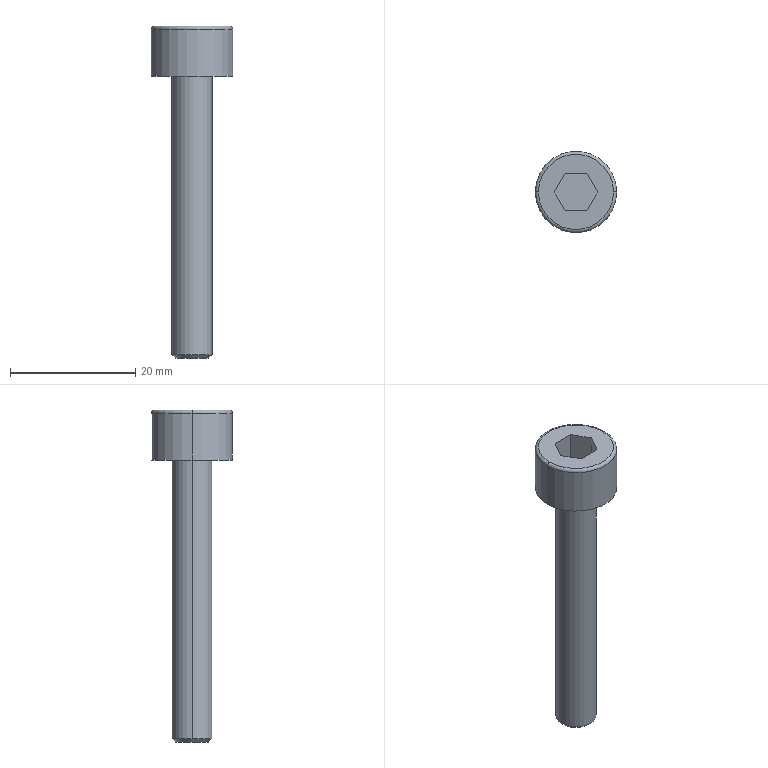Part | CATIA | 1 solid | 18 faces | box 13 x 13 x 53 mm | volume 2318 mm3 | plane 10 | cylinder 4 | torus 2 | cone 2 | commonest cylinder face diameters 6.4 x2 13 x2
STEP:
#1=CARTESIAN_POINT('',(-6.5,0.,0.));
#2=VERTEX_POINT('',#1);
#3=CARTESIAN_POINT('',(6.5,0.,0.));
#4=VERTEX_POINT('',#3);
#5=CARTESIAN_POINT('',(0.,0.,0.));
#6=DIRECTION('',(0.,0.,1.));
#7=AXIS2_PLACEMENT_3D('',#5,#6,$);
#8=CIRCLE('',#7,6.5);
#9=EDGE_CURVE('',#2,#4,#8,.T.);
#10=ORIENTED_EDGE('',*,*,#9,.F.);
#11=CARTESIAN_POINT('',(0.,0.,0.));
#12=DIRECTION('',(0.,0.,1.));
#13=AXIS2_PLACEMENT_3D('',#11,#12,$);
#14=CIRCLE('',#13,6.5);
#15=EDGE_CURVE('',#4,#2,#14,.T.);
#16=ORIENTED_EDGE('',*,*,#15,.F.);
#17=EDGE_LOOP('',(#10,#16));
#18=FACE_OUTER_BOUND('',#17,.T.);
#19=CARTESIAN_POINT('',(-3.2,0.,0.));
#20=VERTEX_POINT('',#19);
#21=CARTESIAN_POINT('',(3.2,0.,0.));
#22=VERTEX_POINT('',#21);
#23=CARTESIAN_POINT('',(0.,0.,0.));
#24=DIRECTION('',(0.,0.,1.));
#25=AXIS2_PLACEMENT_3D('',#23,#24,$);
#26=CIRCLE('',#25,3.2);
#27=EDGE_CURVE('',#20,#22,#26,.F.);
#28=ORIENTED_EDGE('',*,*,#27,.F.);
#29=CARTESIAN_POINT('',(0.,0.,0.));
#30=DIRECTION('',(0.,0.,1.));
#31=AXIS2_PLACEMENT_3D('',#29,#30,$);
#32=CIRCLE('',#31,3.2);
#33=EDGE_CURVE('',#22,#20,#32,.F.);
#34=ORIENTED_EDGE('',*,*,#33,.F.);
#35=EDGE_LOOP('',(#28,#34));
#36=FACE_BOUND('',#35,.T.);
#37=CARTESIAN_POINT('',(0.,0.,0.));
#38=DIRECTION('',(0.,0.,1.));
#39=DIRECTION('',(1.,0.,0.));
#40=AXIS2_PLACEMENT_3D('',#37,#38,#39);
#41=PLANE('',#40);
#42=ADVANCED_FACE('',(#18,#36),#41,.F.);
#43=CARTESIAN_POINT('',(-1.732,-3.,8.));
#44=VERTEX_POINT('',#43);
#45=CARTESIAN_POINT('',(-1.732,-3.,2.));
#46=VERTEX_POINT('',#45);
#47=CARTESIAN_POINT('',(-1.732,-3.,5.));
#48=DIRECTION('',(0.,0.,-1.));
#49=VECTOR('',#48,1.);
#50=LINE('',#47,#49);
#51=EDGE_CURVE('',#44,#46,#50,.T.);
#52=ORIENTED_EDGE('',*,*,#51,.F.);
#53=CARTESIAN_POINT('',(1.732,-3.,8.));
#54=VERTEX_POINT('',#53);
#55=CARTESIAN_POINT('',(0.,-3.,8.));
#56=DIRECTION('',(1.,0.,0.));
#57=VECTOR('',#56,1.);
#58=LINE('',#55,#57);
#59=EDGE_CURVE('',#44,#54,#58,.T.);
#60=ORIENTED_EDGE('',*,*,#59,.T.);
#61=CARTESIAN_POINT('',(1.732,-3.,2.));
#62=VERTEX_POINT('',#61);
#63=CARTESIAN_POINT('',(1.732,-3.,5.));
#64=DIRECTION('',(0.,0.,-1.));
#65=VECTOR('',#64,1.);
#66=LINE('',#63,#65);
#67=EDGE_CURVE('',#54,#62,#66,.T.);
#68=ORIENTED_EDGE('',*,*,#67,.T.);
#69=CARTESIAN_POINT('',(0.,-3.,2.));
#70=DIRECTION('',(1.,0.,0.));
#71=VECTOR('',#70,1.);
#72=LINE('',#69,#71);
#73=EDGE_CURVE('',#46,#62,#72,.T.);
#74=ORIENTED_EDGE('',*,*,#73,.F.);
#75=EDGE_LOOP('',(#52,#60,#68,#74));
#76=FACE_OUTER_BOUND('',#75,.T.);
#77=CARTESIAN_POINT('',(-1.732,-3.,8.));
#78=DIRECTION('',(0.,1.,0.));
#79=DIRECTION('',(1.,0.,0.));
#80=AXIS2_PLACEMENT_3D('',#77,#78,#79);
#81=PLANE('',#80);
#82=ADVANCED_FACE('',(#76),#81,.T.);
#83=CARTESIAN_POINT('',(-3.464,0.,8.));
#84=VERTEX_POINT('',#83);
#85=CARTESIAN_POINT('',(-3.464,0.,2.));
#86=VERTEX_POINT('',#85);
#87=CARTESIAN_POINT('',(-3.464,0.,5.));
#88=DIRECTION('',(0.,0.,-1.));
#89=VECTOR('',#88,1.);
#90=LINE('',#87,#89);
#91=EDGE_CURVE('',#84,#86,#90,.T.);
#92=ORIENTED_EDGE('',*,*,#91,.F.);
#93=CARTESIAN_POINT('',(-2.598,-1.5,8.));
#94=DIRECTION('',(0.5,-0.866,0.));
#95=VECTOR('',#94,1.);
#96=LINE('',#93,#95);
#97=EDGE_CURVE('',#84,#44,#96,.T.);
#98=ORIENTED_EDGE('',*,*,#97,.T.);
#99=ORIENTED_EDGE('',*,*,#51,.T.);
#100=CARTESIAN_POINT('',(-2.598,-1.5,2.));
#101=DIRECTION('',(0.5,-0.866,0.));
#102=VECTOR('',#101,1.);
#103=LINE('',#100,#102);
#104=EDGE_CURVE('',#86,#46,#103,.T.);
#105=ORIENTED_EDGE('',*,*,#104,.F.);
#106=EDGE_LOOP('',(#92,#98,#99,#105));
#107=FACE_OUTER_BOUND('',#106,.T.);
#108=CARTESIAN_POINT('',(-3.464,0.,8.));
#109=DIRECTION('',(0.866,0.5,0.));
#110=DIRECTION('',(0.5,-0.866,0.));
#111=AXIS2_PLACEMENT_3D('',#108,#109,#110);
#112=PLANE('',#111);
#113=ADVANCED_FACE('',(#107),#112,.T.);
#114=ORIENTED_EDGE('',*,*,#67,.F.);
#115=CARTESIAN_POINT('',(3.464,0.,8.));
#116=VERTEX_POINT('',#115);
#117=CARTESIAN_POINT('',(2.598,-1.5,8.));
#118=DIRECTION('',(0.5,0.866,0.));
#119=VECTOR('',#118,1.);
#120=LINE('',#117,#119);
#121=EDGE_CURVE('',#54,#116,#120,.T.);
#122=ORIENTED_EDGE('',*,*,#121,.T.);
#123=CARTESIAN_POINT('',(3.464,0.,2.));
#124=VERTEX_POINT('',#123);
#125=CARTESIAN_POINT('',(3.464,0.,5.));
#126=DIRECTION('',(0.,0.,-1.));
#127=VECTOR('',#126,1.);
#128=LINE('',#125,#127);
#129=EDGE_CURVE('',#116,#124,#128,.T.);
#130=ORIENTED_EDGE('',*,*,#129,.T.);
#131=CARTESIAN_POINT('',(2.598,-1.5,2.));
#132=DIRECTION('',(0.5,0.866,0.));
#133=VECTOR('',#132,1.);
#134=LINE('',#131,#133);
#135=EDGE_CURVE('',#62,#124,#134,.T.);
#136=ORIENTED_EDGE('',*,*,#135,.F.);
#137=EDGE_LOOP('',(#114,#122,#130,#136));
#138=FACE_OUTER_BOUND('',#137,.T.);
#139=CARTESIAN_POINT('',(1.732,-3.,8.));
#140=DIRECTION('',(-0.866,0.5,0.));
#141=DIRECTION('',(0.5,0.866,0.));
#142=AXIS2_PLACEMENT_3D('',#139,#140,#141);
#143=PLANE('',#142);
#144=ADVANCED_FACE('',(#138),#143,.T.);
#145=CARTESIAN_POINT('',(1.732,3.,2.));
#146=VERTEX_POINT('',#145);
#147=CARTESIAN_POINT('',(-1.732,3.,2.));
#148=VERTEX_POINT('',#147);
#149=CARTESIAN_POINT('',(0.,3.,2.));
#150=DIRECTION('',(-1.,0.,0.));
#151=VECTOR('',#150,1.);
#152=LINE('',#149,#151);
#153=EDGE_CURVE('',#146,#148,#152,.T.);
#154=ORIENTED_EDGE('',*,*,#153,.T.);
#155=CARTESIAN_POINT('',(-2.598,1.5,2.));
#156=DIRECTION('',(-0.5,-0.866,0.));
#157=VECTOR('',#156,1.);
#158=LINE('',#155,#157);
#159=EDGE_CURVE('',#148,#86,#158,.T.);
#160=ORIENTED_EDGE('',*,*,#159,.T.);
#161=ORIENTED_EDGE('',*,*,#104,.T.);
#162=ORIENTED_EDGE('',*,*,#73,.T.);
#163=ORIENTED_EDGE('',*,*,#135,.T.);
#164=CARTESIAN_POINT('',(2.598,1.5,2.));
#165=DIRECTION('',(-0.5,0.866,0.));
#166=VECTOR('',#165,1.);
#167=LINE('',#164,#166);
#168=EDGE_CURVE('',#124,#146,#167,.T.);
#169=ORIENTED_EDGE('',*,*,#168,.T.);
#170=EDGE_LOOP('',(#154,#160,#161,#162,#163,#169));
#171=FACE_OUTER_BOUND('',#170,.T.);
#172=CARTESIAN_POINT('',(0.,0.,2.));
#173=DIRECTION('',(0.,0.,1.));
#174=DIRECTION('',(1.,0.,0.));
#175=AXIS2_PLACEMENT_3D('',#172,#173,#174);
#176=PLANE('',#175);
#177=ADVANCED_FACE('',(#171),#176,.T.);
#178=CARTESIAN_POINT('',(-1.732,3.,8.));
#179=VERTEX_POINT('',#178);
#180=CARTESIAN_POINT('',(-1.732,3.,5.));
#181=DIRECTION('',(0.,0.,-1.));
#182=VECTOR('',#181,1.);
#183=LINE('',#180,#182);
#184=EDGE_CURVE('',#179,#148,#183,.T.);
#185=ORIENTED_EDGE('',*,*,#184,.F.);
#186=CARTESIAN_POINT('',(-2.598,1.5,8.));
#187=DIRECTION('',(-0.5,-0.866,0.));
#188=VECTOR('',#187,1.);
#189=LINE('',#186,#188);
#190=EDGE_CURVE('',#179,#84,#189,.T.);
#191=ORIENTED_EDGE('',*,*,#190,.T.);
#192=ORIENTED_EDGE('',*,*,#91,.T.);
#193=ORIENTED_EDGE('',*,*,#159,.F.);
#194=EDGE_LOOP('',(#185,#191,#192,#193));
#195=FACE_OUTER_BOUND('',#194,.T.);
#196=CARTESIAN_POINT('',(-1.732,3.,8.));
#197=DIRECTION('',(0.866,-0.5,0.));
#198=DIRECTION('',(-0.5,-0.866,0.));
#199=AXIS2_PLACEMENT_3D('',#196,#197,#198);
#200=PLANE('',#199);
#201=ADVANCED_FACE('',(#195),#200,.T.);
#202=ORIENTED_EDGE('',*,*,#129,.F.);
#203=CARTESIAN_POINT('',(1.732,3.,8.));
#204=VERTEX_POINT('',#203);
#205=CARTESIAN_POINT('',(2.598,1.5,8.));
#206=DIRECTION('',(-0.5,0.866,0.));
#207=VECTOR('',#206,1.);
#208=LINE('',#205,#207);
#209=EDGE_CURVE('',#116,#204,#208,.T.);
#210=ORIENTED_EDGE('',*,*,#209,.T.);
#211=CARTESIAN_POINT('',(1.732,3.,5.));
#212=DIRECTION('',(0.,0.,-1.));
#213=VECTOR('',#212,1.);
#214=LINE('',#211,#213);
#215=EDGE_CURVE('',#204,#146,#214,.T.);
#216=ORIENTED_EDGE('',*,*,#215,.T.);
#217=ORIENTED_EDGE('',*,*,#168,.F.);
#218=EDGE_LOOP('',(#202,#210,#216,#217));
#219=FACE_OUTER_BOUND('',#218,.T.);
#220=CARTESIAN_POINT('',(3.464,0.,8.));
#221=DIRECTION('',(-0.866,-0.5,0.));
#222=DIRECTION('',(-0.5,0.866,0.));
#223=AXIS2_PLACEMENT_3D('',#220,#221,#222);
#224=PLANE('',#223);
#225=ADVANCED_FACE('',(#219),#224,.T.);
#226=ORIENTED_EDGE('',*,*,#215,.F.);
#227=CARTESIAN_POINT('',(0.,3.,8.));
#228=DIRECTION('',(-1.,0.,0.));
#229=VECTOR('',#228,1.);
#230=LINE('',#227,#229);
#231=EDGE_CURVE('',#204,#179,#230,.T.);
#232=ORIENTED_EDGE('',*,*,#231,.T.);
#233=ORIENTED_EDGE('',*,*,#184,.T.);
#234=ORIENTED_EDGE('',*,*,#153,.F.);
#235=EDGE_LOOP('',(#226,#232,#233,#234));
#236=FACE_OUTER_BOUND('',#235,.T.);
#237=CARTESIAN_POINT('',(1.732,3.,8.));
#238=DIRECTION('',(0.,-1.,0.));
#239=DIRECTION('',(-1.,0.,0.));
#240=AXIS2_PLACEMENT_3D('',#237,#238,#239);
#241=PLANE('',#240);
#242=ADVANCED_FACE('',(#236),#241,.T.);
#243=CARTESIAN_POINT('',(-6.,0.000000322,8.));
#244=VERTEX_POINT('',#243);
#245=CARTESIAN_POINT('',(6.,0.,8.));
#246=VERTEX_POINT('',#245);
#247=CARTESIAN_POINT('',(0.,0.,8.));
#248=DIRECTION('',(0.,0.,1.));
#249=AXIS2_PLACEMENT_3D('',#247,#248,$);
#250=CIRCLE('',#249,6.);
#251=EDGE_CURVE('',#244,#246,#250,.T.);
#252=ORIENTED_EDGE('',*,*,#251,.T.);
#253=CARTESIAN_POINT('',(0.,0.,8.));
#254=DIRECTION('',(0.,0.,1.));
#255=AXIS2_PLACEMENT_3D('',#253,#254,$);
#256=CIRCLE('',#255,6.);
#257=EDGE_CURVE('',#246,#244,#256,.T.);
#258=ORIENTED_EDGE('',*,*,#257,.T.);
#259=EDGE_LOOP('',(#252,#258));
#260=FACE_OUTER_BOUND('',#259,.T.);
#261=ORIENTED_EDGE('',*,*,#121,.F.);
#262=ORIENTED_EDGE('',*,*,#59,.F.);
#263=ORIENTED_EDGE('',*,*,#97,.F.);
#264=ORIENTED_EDGE('',*,*,#190,.F.);
#265=ORIENTED_EDGE('',*,*,#231,.F.);
#266=ORIENTED_EDGE('',*,*,#209,.F.);
#267=EDGE_LOOP('',(#261,#262,#263,#264,#265,#266));
#268=FACE_BOUND('',#267,.T.);
#269=CARTESIAN_POINT('',(0.,0.,8.));
#270=DIRECTION('',(0.,0.,1.));
#271=DIRECTION('',(1.,0.,0.));
#272=AXIS2_PLACEMENT_3D('',#269,#270,#271);
#273=PLANE('',#272);
#274=ADVANCED_FACE('',(#260,#268),#273,.T.);
#275=CARTESIAN_POINT('',(-6.5,0.,7.5));
#276=VERTEX_POINT('',#275);
#277=CARTESIAN_POINT('',(-6.5,0.,4.));
#278=DIRECTION('',(0.,0.,1.));
#279=VECTOR('',#278,1.);
#280=LINE('',#277,#279);
#281=EDGE_CURVE('',#2,#276,#280,.T.);
#282=ORIENTED_EDGE('',*,*,#281,.F.);
#283=ORIENTED_EDGE('',*,*,#9,.T.);
#284=CARTESIAN_POINT('',(6.5,0.,7.5));
#285=VERTEX_POINT('',#284);
#286=CARTESIAN_POINT('',(6.5,0.,4.));
#287=DIRECTION('',(0.,0.,1.));
#288=VECTOR('',#287,1.);
#289=LINE('',#286,#288);
#290=EDGE_CURVE('',#4,#285,#289,.T.);
#291=ORIENTED_EDGE('',*,*,#290,.T.);
#292=CARTESIAN_POINT('',(0.,0.,7.5));
#293=DIRECTION('',(0.,0.,1.));
#294=AXIS2_PLACEMENT_3D('',#292,#293,$);
#295=CIRCLE('',#294,6.5);
#296=EDGE_CURVE('',#276,#285,#295,.T.);
#297=ORIENTED_EDGE('',*,*,#296,.F.);
#298=EDGE_LOOP('',(#282,#283,#291,#297));
#299=FACE_OUTER_BOUND('',#298,.T.);
#300=CARTESIAN_POINT('',(0.,0.,4.));
#301=DIRECTION('',(0.,0.,1.));
#302=DIRECTION('',(1.,0.,0.));
#303=AXIS2_PLACEMENT_3D('',#300,#301,#302);
#304=CYLINDRICAL_SURFACE('',#303,6.5);
#305=ADVANCED_FACE('',(#299),#304,.T.);
#306=ORIENTED_EDGE('',*,*,#290,.F.);
#307=ORIENTED_EDGE('',*,*,#15,.T.);
#308=ORIENTED_EDGE('',*,*,#281,.T.);
#309=CARTESIAN_POINT('',(0.,0.,7.5));
#310=DIRECTION('',(0.,0.,1.));
#311=AXIS2_PLACEMENT_3D('',#309,#310,$);
#312=CIRCLE('',#311,6.5);
#313=EDGE_CURVE('',#285,#276,#312,.T.);
#314=ORIENTED_EDGE('',*,*,#313,.F.);
#315=EDGE_LOOP('',(#306,#307,#308,#314));
#316=FACE_OUTER_BOUND('',#315,.T.);
#317=ADVANCED_FACE('',(#316),#304,.T.);
#318=CARTESIAN_POINT('',(-6.,0.,7.5));
#319=DIRECTION('',(0.,1.,0.));
#320=AXIS2_PLACEMENT_3D('',#318,#319,$);
#321=CIRCLE('',#320,0.5);
#322=EDGE_CURVE('',#244,#276,#321,.F.);
#323=ORIENTED_EDGE('',*,*,#322,.T.);
#324=ORIENTED_EDGE('',*,*,#296,.T.);
#325=CARTESIAN_POINT('',(6.,0.,7.5));
#326=DIRECTION('',(0.,-1.,0.));
#327=AXIS2_PLACEMENT_3D('',#325,#326,$);
#328=CIRCLE('',#327,0.5);
#329=EDGE_CURVE('',#246,#285,#328,.F.);
#330=ORIENTED_EDGE('',*,*,#329,.F.);
#331=ORIENTED_EDGE('',*,*,#251,.F.);
#332=EDGE_LOOP('',(#323,#324,#330,#331));
#333=FACE_OUTER_BOUND('',#332,.T.);
#334=CARTESIAN_POINT('',(0.,0.,7.5));
#335=DIRECTION('',(0.,0.,1.));
#336=DIRECTION('',(-0.9461,0.3239,0.));
#337=AXIS2_PLACEMENT_3D('',#334,#335,#336);
#338=TOROIDAL_SURFACE('',#337,6.,0.5);
#339=ADVANCED_FACE('',(#333),#338,.T.);
#340=ORIENTED_EDGE('',*,*,#329,.T.);
#341=ORIENTED_EDGE('',*,*,#313,.T.);
#342=ORIENTED_EDGE('',*,*,#322,.F.);
#343=ORIENTED_EDGE('',*,*,#257,.F.);
#344=EDGE_LOOP('',(#340,#341,#342,#343));
#345=FACE_OUTER_BOUND('',#344,.T.);
#346=CARTESIAN_POINT('',(0.,0.,7.5));
#347=DIRECTION('',(0.,0.,1.));
#348=DIRECTION('',(1.,0.,0.));
#349=AXIS2_PLACEMENT_3D('',#346,#347,#348);
#350=TOROIDAL_SURFACE('',#349,6.,0.5);
#351=ADVANCED_FACE('',(#345),#350,.T.);
#352=CARTESIAN_POINT('',(3.2,0.,-44.5));
#353=VERTEX_POINT('',#352);
#354=CARTESIAN_POINT('',(3.2,0.,-22.5));
#355=DIRECTION('',(0.,0.,-1.));
#356=VECTOR('',#355,1.);
#357=LINE('',#354,#356);
#358=EDGE_CURVE('',#22,#353,#357,.T.);
#359=ORIENTED_EDGE('',*,*,#358,.F.);
#360=ORIENTED_EDGE('',*,*,#33,.T.);
#361=CARTESIAN_POINT('',(-3.2,0.,-44.5));
#362=VERTEX_POINT('',#361);
#363=CARTESIAN_POINT('',(-3.2,0.,-22.5));
#364=DIRECTION('',(0.,0.,-1.));
#365=VECTOR('',#364,1.);
#366=LINE('',#363,#365);
#367=EDGE_CURVE('',#20,#362,#366,.T.);
#368=ORIENTED_EDGE('',*,*,#367,.T.);
#369=CARTESIAN_POINT('',(0.,0.,-44.5));
#370=DIRECTION('',(0.,0.,-1.));
#371=AXIS2_PLACEMENT_3D('',#369,#370,$);
#372=CIRCLE('',#371,3.2);
#373=EDGE_CURVE('',#353,#362,#372,.T.);
#374=ORIENTED_EDGE('',*,*,#373,.F.);
#375=EDGE_LOOP('',(#359,#360,#368,#374));
#376=FACE_OUTER_BOUND('',#375,.T.);
#377=CARTESIAN_POINT('',(0.,0.,-22.5));
#378=DIRECTION('',(0.,0.,-1.));
#379=DIRECTION('',(1.,0.,0.));
#380=AXIS2_PLACEMENT_3D('',#377,#378,#379);
#381=CYLINDRICAL_SURFACE('',#380,3.2);
#382=ADVANCED_FACE('',(#376),#381,.T.);
#383=ORIENTED_EDGE('',*,*,#367,.F.);
#384=ORIENTED_EDGE('',*,*,#27,.T.);
#385=ORIENTED_EDGE('',*,*,#358,.T.);
#386=CARTESIAN_POINT('',(0.,0.,-44.5));
#387=DIRECTION('',(0.,0.,-1.));
#388=AXIS2_PLACEMENT_3D('',#386,#387,$);
#389=CIRCLE('',#388,3.2);
#390=EDGE_CURVE('',#362,#353,#389,.T.);
#391=ORIENTED_EDGE('',*,*,#390,.F.);
#392=EDGE_LOOP('',(#383,#384,#385,#391));
#393=FACE_OUTER_BOUND('',#392,.T.);
#394=ADVANCED_FACE('',(#393),#381,.T.);
#395=CARTESIAN_POINT('',(-2.7,-0.000000824,-45.));
#396=VERTEX_POINT('',#395);
#397=CARTESIAN_POINT('',(2.7,0.,-45.));
#398=VERTEX_POINT('',#397);
#399=CARTESIAN_POINT('',(0.,0.,-45.));
#400=DIRECTION('',(0.,0.,-1.));
#401=AXIS2_PLACEMENT_3D('',#399,#400,$);
#402=CIRCLE('',#401,2.7);
#403=EDGE_CURVE('',#396,#398,#402,.T.);
#404=ORIENTED_EDGE('',*,*,#403,.T.);
#405=CARTESIAN_POINT('',(0.,0.,-45.));
#406=DIRECTION('',(0.,0.,-1.));
#407=AXIS2_PLACEMENT_3D('',#405,#406,$);
#408=CIRCLE('',#407,2.7);
#409=EDGE_CURVE('',#398,#396,#408,.T.);
#410=ORIENTED_EDGE('',*,*,#409,.T.);
#411=EDGE_LOOP('',(#404,#410));
#412=FACE_OUTER_BOUND('',#411,.T.);
#413=CARTESIAN_POINT('',(0.,0.,-45.));
#414=DIRECTION('',(0.,0.,-1.));
#415=DIRECTION('',(1.,0.,0.));
#416=AXIS2_PLACEMENT_3D('',#413,#414,#415);
#417=PLANE('',#416);
#418=ADVANCED_FACE('',(#412),#417,.T.);
#419=CARTESIAN_POINT('',(-2.95,0.,-44.75));
#420=DIRECTION('',(-0.7071,0.,0.7071));
#421=VECTOR('',#420,1.);
#422=LINE('',#419,#421);
#423=EDGE_CURVE('',#396,#362,#422,.T.);
#424=ORIENTED_EDGE('',*,*,#423,.T.);
#425=ORIENTED_EDGE('',*,*,#390,.T.);
#426=CARTESIAN_POINT('',(2.95,0.,-44.75));
#427=DIRECTION('',(0.7071,0.,0.7071));
#428=VECTOR('',#427,1.);
#429=LINE('',#426,#428);
#430=EDGE_CURVE('',#398,#353,#429,.T.);
#431=ORIENTED_EDGE('',*,*,#430,.F.);
#432=ORIENTED_EDGE('',*,*,#403,.F.);
#433=EDGE_LOOP('',(#424,#425,#431,#432));
#434=FACE_OUTER_BOUND('',#433,.T.);
#435=CARTESIAN_POINT('',(0.,0.,-47.7));
#436=DIRECTION('',(0.,0.,1.));
#437=DIRECTION('',(-0.9723,-0.2337,0.));
#438=AXIS2_PLACEMENT_3D('',#435,#436,#437);
#439=CONICAL_SURFACE('',#438,0.,0.7854);
#440=ADVANCED_FACE('',(#434),#439,.T.);
#441=ORIENTED_EDGE('',*,*,#430,.T.);
#442=ORIENTED_EDGE('',*,*,#373,.T.);
#443=ORIENTED_EDGE('',*,*,#423,.F.);
#444=ORIENTED_EDGE('',*,*,#409,.F.);
#445=EDGE_LOOP('',(#441,#442,#443,#444));
#446=FACE_OUTER_BOUND('',#445,.T.);
#447=CARTESIAN_POINT('',(0.,0.,-47.7));
#448=DIRECTION('',(0.,0.,1.));
#449=DIRECTION('',(1.,0.,0.));
#450=AXIS2_PLACEMENT_3D('',#447,#448,#449);
#451=CONICAL_SURFACE('',#450,0.,0.7854);
#452=ADVANCED_FACE('',(#446),#451,.T.);
#453=CLOSED_SHELL('',(#42,#82,#113,#144,#177,#201,#225,#242,#274,#305,#317,#339,#351,#382,#394,#418,#440,#452));
#454=MANIFOLD_SOLID_BREP('',#453);
#455=(LENGTH_UNIT()NAMED_UNIT(*)SI_UNIT(.MILLI.,.METRE.));
#456=UNCERTAINTY_MEASURE_WITH_UNIT(LENGTH_MEASURE(0.005),#455,'','');
#457=(NAMED_UNIT(*)PLANE_ANGLE_UNIT()SI_UNIT($,.RADIAN.));
#458=(NAMED_UNIT(*)SI_UNIT($,.STERADIAN.)SOLID_ANGLE_UNIT());
#459=(GEOMETRIC_REPRESENTATION_CONTEXT(3)GLOBAL_UNCERTAINTY_ASSIGNED_CONTEXT((#456))GLOBAL_UNIT_ASSIGNED_CONTEXT((#455,#457,#458))REPRESENTATION_CONTEXT('',''));
#460=ADVANCED_BREP_SHAPE_REPRESENTATION('',(#454),#459);